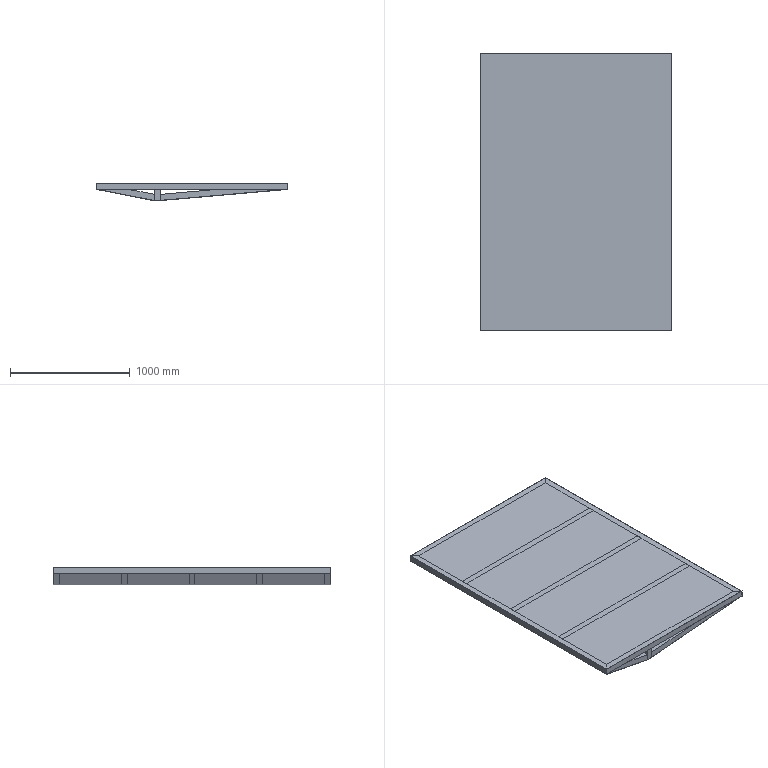Part | SolidWorks | features WeldCornerFeat 2, 3DProfileFeature 1, BossThin 1, WeldMemberFeat 1, WeldmentFeature 1 | 24 solids | 150 faces | box 1604 x 2324 x 150.468 mm | volume 66441316 mm3 | plane 150